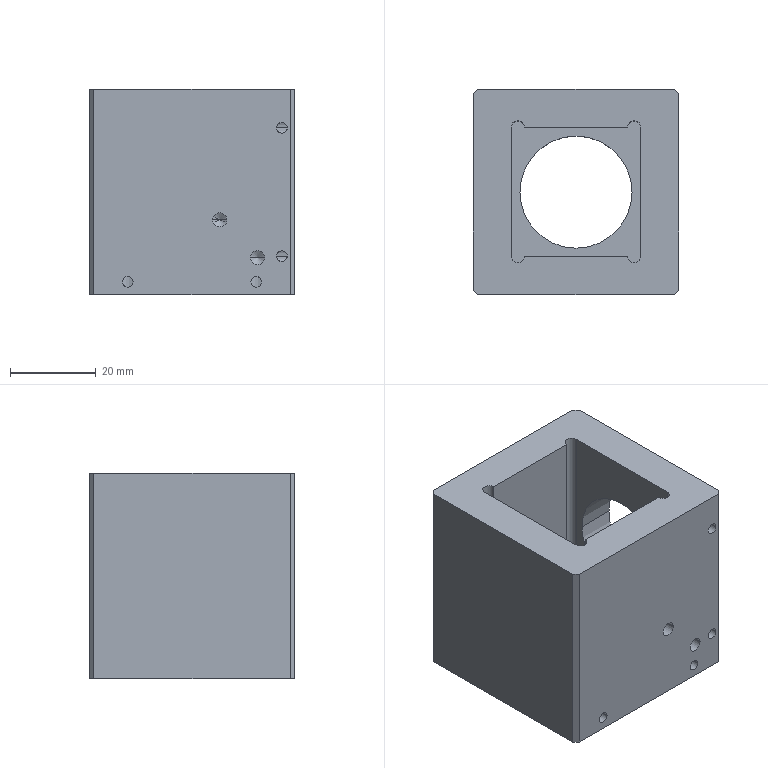NC program | NX | posted with a generic post | part box 48 x 48 x 48 mm
Whole program:
N10 G17 G21 G94 G90
(DRILLING_COPY_1_COPY , TOOL : D6A45)
N12 T01 M6
N14 G54
N16 G17 G0 G90 X21. Y-15. B0. C0. S5000 M3
N18 G43 Z30. H1
N20 G94 G81 G98 Z-1. F350. R3.
N22 X15.339 Y-2.339
N24 X6.5 Y6.5
N26 X21. Y15.
N28 X15. Y21.
N30 X-2.339 Y15.339
N32 X-15. Y21.
N34 G80
N36 G0 X-15. Y21. Z30.
N38 M5
(DRILLING_COPY_1_COPY_1_1_COPY_1_COPY , TOOL : 2.5ZT)
N40 T02 M6
N42 G54
N44 G17 G0 G90 X21. Y-15. B0. C0. S2000 M3
N46 G43 Z30. H2
N48 G94 G83 G98 Z-49.751 F80. Q2. R3.
N50 Y15.
N52 X15. Y21.
N54 X-15.
N56 G80
N58 G0 X-15. Y21. Z30.
N60 M5
(DRILLING_COPY_1_COPY_1_1_COPY_1_1 , TOOL : 3.3ZT)
N62 T03 M6
N64 G54
N66 G17 G0 G90 X15.339 Y-2.339 B0. C0. S2000 M3
N68 G43 Z30. H3
N70 G94 G83 G98 Z-6.991 F200. Q2. R3.
N72 X6.5 Y6.5
N74 X-2.339 Y15.339
N76 G80
N78 G0 X-2.339 Y15.339 Z30.
N80 M5
(PLANAR_MILL_COPY_COPY_COPY_COPY_COPY_COPY_1_COPY_1_COPY_COPY_COPY , TOOL : D6A45)
N82 T01 M6
N84 G54
N86 G17 G0 G90 X21.373 Y-14.756 B0. C0. S9500 M3
N88 G43 Z30. H1
N90 Z0.5
N92 G94 G1 X21.167 Y-14.55 Z0.422 F1250.
N94 X20.833 Z0.332
N96 X20.55 Y-14.833 Z0.225
N98 Y-15.167 Z0.136
N100 X20.833 Y-15.45 Z0.028
N102 X21.167 Z-0.061
N104 X21.45 Y-15.167 Z-0.168
N106 Y-14.833 Z-0.258
N108 X21.167 Y-14.55 Z-0.365
N110 X20.833 Z-0.455
N112 X20.55 Y-14.833 Z-0.562
N114 Y-15.167 Z-0.651
N116 X20.833 Y-15.45 Z-0.759
N118 X21.167 Z-0.848
N120 X21.45 Y-15.167 Z-0.955
N122 Y-15. Z-1.
N124 G3 X21. Y-14.55 R0.45
N126 X21.45 Y-15. R-0.45
N128 X21.383 Y-14.75 R0.5
N130 G1 Z0.5
N132 G0 Z30.
N134 X16.189 Y-2.471
N136 Z0.5
N138 G1 Y-2.111 Z0.404
N140 X15.961 Y-1.717 Z0.282
N142 X15.567 Y-1.489 Z0.16
N144 X15.111 Z0.037
N146 X14.717 Y-1.717 Z-0.085
N148 X14.489 Y-2.111 Z-0.207
N150 Y-2.567 Z-0.329
N152 X14.717 Y-2.961 Z-0.451
N154 X15.111 Y-3.189 Z-0.573
N156 X15.567 Z-0.695
N158 X15.961 Y-2.961 Z-0.817
N160 X16.189 Y-2.567 Z-0.939
N162 Y-2.339 Z-1.
N164 G3 X15.339 Y-1.489 R0.85
N166 X16.189 Y-2.339 R-0.85
N168 X15.939 Y-1.906 R0.5
N170 G1 Z0.5
N172 G0 Z30.
N174 X7.35 Y6.368
N176 Z0.5
N178 G1 Y6.728 Z0.404
N180 X7.122 Y7.122 Z0.282
N182 X6.728 Y7.35 Z0.16
N184 X6.272 Z0.037
N186 X5.878 Y7.122 Z-0.085
N188 X5.65 Y6.728 Z-0.207
N190 Y6.272 Z-0.329
N192 X5.878 Y5.878 Z-0.451
N194 X6.272 Y5.65 Z-0.573
N196 X6.728 Z-0.695
N198 X7.122 Y5.878 Z-0.817
N200 X7.35 Y6.272 Z-0.939
N202 Y6.5 Z-1.
N204 G3 X6.5 Y7.35 R0.85
N206 X7.35 Y6.5 R-0.85
N208 X7.1 Y6.933 R0.5
N210 G1 Z0.5
N212 G0 Z30.
N214 X21.373 Y15.244
N216 Z0.5
N218 G1 X21.167 Y15.45 Z0.422
N220 X20.833 Z0.332
N222 X20.55 Y15.167 Z0.225
N224 Y14.833 Z0.136
N226 X20.833 Y14.55 Z0.028
N228 X21.167 Z-0.061
N230 X21.45 Y14.833 Z-0.168
N232 Y15.167 Z-0.258
N234 X21.167 Y15.45 Z-0.365
N236 X20.833 Z-0.455
N238 X20.55 Y15.167 Z-0.562
N240 Y14.833 Z-0.651
N242 X20.833 Y14.55 Z-0.759
N244 X21.167 Z-0.848
N246 X21.45 Y14.833 Z-0.955
N248 Y15. Z-1.
N250 G3 X21. Y15.45 R0.45
N252 X21.45 Y15. R-0.45
N254 X21.383 Y15.25 R0.5
N256 G1 Z0.5
N258 G0 Z30.
N260 X14.756 Y21.373
N262 Z0.5
N264 G1 X14.55 Y21.167 Z0.422
N266 Y20.833 Z0.332
N268 X14.833 Y20.55 Z0.225
N270 X15.167 Z0.136
N272 X15.45 Y20.833 Z0.028
N274 Y21.167 Z-0.061
N276 X15.167 Y21.45 Z-0.168
N278 X14.833 Z-0.258
N280 X14.55 Y21.167 Z-0.365
N282 Y20.833 Z-0.455
N284 X14.833 Y20.55 Z-0.562
N286 X15.167 Z-0.651
N288 X15.45 Y20.833 Z-0.759
N290 Y21.167 Z-0.848
N292 X15.167 Y21.45 Z-0.955
N294 X15. Z-1.
N296 G3 X14.55 Y21. R0.45
N298 X15. Y21.45 R-0.45
N300 X14.75 Y21.383 R0.5
N302 G1 Z0.5
N304 G0 Z30.
N306 X-2.207 Y16.189
N308 Z0.5
N310 G1 X-2.567 Z0.404
N312 X-2.961 Y15.961 Z0.282
N314 X-3.189 Y15.567 Z0.16
N316 Y15.111 Z0.037
N318 X-2.961 Y14.717 Z-0.085
N320 X-2.567 Y14.489 Z-0.207
N322 X-2.111 Z-0.329
N324 X-1.717 Y14.717 Z-0.451
N326 X-1.489 Y15.111 Z-0.573
N328 Y15.567 Z-0.695
N330 X-1.717 Y15.961 Z-0.817
N332 X-2.111 Y16.189 Z-0.939
N334 X-2.339 Z-1.
N336 G3 X-3.189 Y15.339 R0.85
N338 X-2.339 Y16.189 R-0.85
N340 X-2.772 Y15.939 R0.5
N342 G1 Z0.5
N344 G0 Z30.
N346 X-15.244 Y21.373
N348 Z0.5
N350 G1 X-15.45 Y21.167 Z0.422
N352 Y20.833 Z0.332
N354 X-15.167 Y20.55 Z0.225
N356 X-14.833 Z0.136
N358 X-14.55 Y20.833 Z0.028
N360 Y21.167 Z-0.061
N362 X-14.833 Y21.45 Z-0.168
N364 X-15.167 Z-0.258
N366 X-15.45 Y21.167 Z-0.365
N368 Y20.833 Z-0.455
N370 X-15.167 Y20.55 Z-0.562
N372 X-14.833 Z-0.651
N374 X-14.55 Y20.833 Z-0.759
N376 Y21.167 Z-0.848
N378 X-14.833 Y21.45 Z-0.955
N380 X-15. Z-1.
N382 G3 X-15.45 Y21. R0.45
N384 X-15. Y21.45 R-0.45
N386 X-15.25 Y21.383 R0.5
N388 G1 Z0.5
N390 G0 Z30.
N392 M5
N394 M2